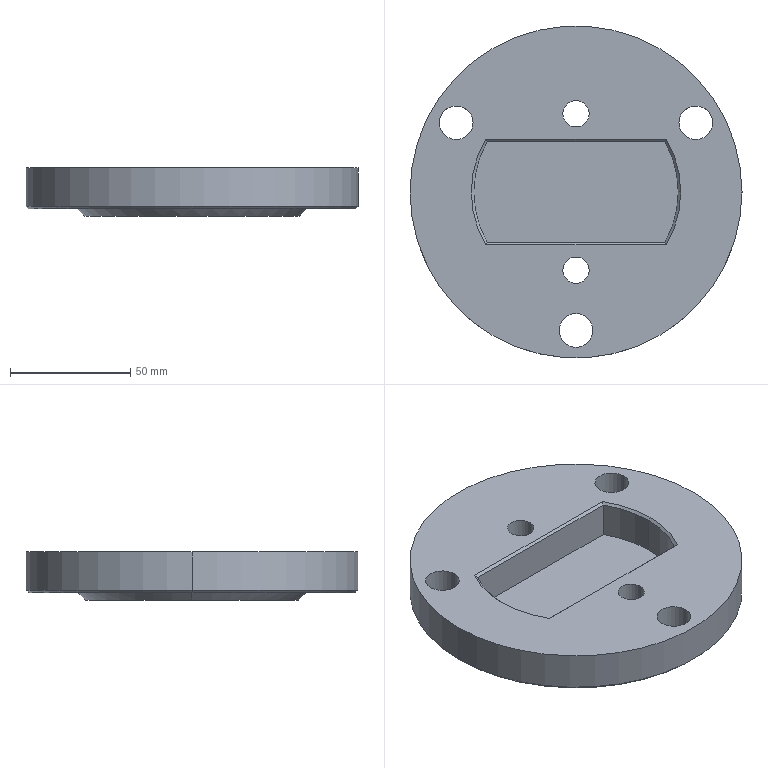Part | SolidWorks | features Chamfer 3, ICE 3, 3DProfileFeature 1, Extrusion 1, HoleWzd 1 | 1 solid | 36 faces | box 138 x 138 x 20 mm | volume 204024 mm3 | cylinder 19 | plane 10 | cone 7 | commonest cylinder face diameters 14 x6 11 x4 18 x4 85 x3 138 x2
STEP:
#1=CARTESIAN_POINT('',(42.5,0.,19.));
#2=VERTEX_POINT('',#1);
#3=CARTESIAN_POINT('',(36.949,21.,19.));
#4=VERTEX_POINT('',#3);
#5=CARTESIAN_POINT('',(0.,0.,19.));
#6=DIRECTION('',(0.,0.,1.));
#7=DIRECTION('',(1.,0.,0.));
#8=AXIS2_PLACEMENT_3D('',#5,#6,#7);
#9=CIRCLE('',#8,42.5);
#10=EDGE_CURVE('',#2,#4,#9,.T.);
#11=ORIENTED_EDGE('',*,*,#10,.F.);
#12=CARTESIAN_POINT('',(43.5,0.,20.));
#13=VERTEX_POINT('',#12);
#14=CARTESIAN_POINT('',(42.5,0.,19.));
#15=DIRECTION('',(0.7071,0.,0.7071));
#16=VECTOR('',#15,1000.);
#17=LINE('',#14,#16);
#18=EDGE_CURVE('',#2,#13,#17,.T.);
#19=ORIENTED_EDGE('',*,*,#18,.T.);
#20=CARTESIAN_POINT('',(37.527,22.,20.));
#21=VERTEX_POINT('',#20);
#22=CARTESIAN_POINT('',(0.,0.,20.));
#23=DIRECTION('',(0.,0.,-1.));
#24=DIRECTION('',(1.,0.,0.));
#25=AXIS2_PLACEMENT_3D('',#22,#23,#24);
#26=CIRCLE('',#25,43.5);
#27=EDGE_CURVE('',#21,#13,#26,.T.);
#28=ORIENTED_EDGE('',*,*,#27,.F.);
#29=CARTESIAN_POINT('',(37.527,22.,20.));
#30=CARTESIAN_POINT('',(37.335,21.666,19.666));
#31=CARTESIAN_POINT('',(37.143,21.333,19.333));
#32=CARTESIAN_POINT('',(36.949,21.,19.));
#33=B_SPLINE_CURVE_WITH_KNOTS('',3,(#29,#30,#31,#32),.UNSPECIFIED.,.F.,.F.,(4,4),(0.,0.001528),.UNSPECIFIED.);
#34=EDGE_CURVE('',#21,#4,#33,.T.);
#35=ORIENTED_EDGE('',*,*,#34,.T.);
#36=EDGE_LOOP('',(#11,#19,#28,#35));
#37=FACE_OUTER_BOUND('',#36,.T.);
#38=CARTESIAN_POINT('',(0.,0.,19.));
#39=DIRECTION('',(0.,0.,1.));
#40=DIRECTION('',(1.,0.,0.));
#41=AXIS2_PLACEMENT_3D('',#38,#39,#40);
#42=CONICAL_SURFACE('',#41,42.5,0.7854);
#43=ADVANCED_FACE('',(#37),#42,.F.);
#44=CARTESIAN_POINT('',(9.,32.5,11.));
#45=VERTEX_POINT('',#44);
#46=CARTESIAN_POINT('',(-9.,32.5,11.));
#47=VERTEX_POINT('',#46);
#48=CARTESIAN_POINT('',(0.,32.5,11.));
#49=DIRECTION('',(0.,0.,-1.));
#50=DIRECTION('',(-1.,0.,0.));
#51=AXIS2_PLACEMENT_3D('',#48,#49,#50);
#52=CIRCLE('',#51,9.);
#53=EDGE_CURVE('',#45,#47,#52,.T.);
#54=ORIENTED_EDGE('',*,*,#53,.F.);
#55=CARTESIAN_POINT('',(9.,32.5,0.));
#56=VERTEX_POINT('',#55);
#57=CARTESIAN_POINT('',(9.,32.5,0.));
#58=DIRECTION('',(0.,0.,-1.));
#59=VECTOR('',#58,1000.);
#60=LINE('',#57,#59);
#61=EDGE_CURVE('',#45,#56,#60,.T.);
#62=ORIENTED_EDGE('',*,*,#61,.T.);
#63=CARTESIAN_POINT('',(-9.,32.5,0.));
#64=VERTEX_POINT('',#63);
#65=CARTESIAN_POINT('',(0.,32.5,0.));
#66=DIRECTION('',(0.,0.,-1.));
#67=DIRECTION('',(-1.,0.,0.));
#68=AXIS2_PLACEMENT_3D('',#65,#66,#67);
#69=CIRCLE('',#68,9.);
#70=EDGE_CURVE('',#56,#64,#69,.T.);
#71=ORIENTED_EDGE('',*,*,#70,.T.);
#72=CARTESIAN_POINT('',(-9.,32.5,0.));
#73=DIRECTION('',(0.,0.,-1.));
#74=VECTOR('',#73,1000.);
#75=LINE('',#72,#74);
#76=EDGE_CURVE('',#47,#64,#75,.T.);
#77=ORIENTED_EDGE('',*,*,#76,.F.);
#78=EDGE_LOOP('',(#54,#62,#71,#77));
#79=FACE_OUTER_BOUND('',#78,.T.);
#80=CARTESIAN_POINT('',(0.,32.5,0.));
#81=DIRECTION('',(0.,0.,-1.));
#82=DIRECTION('',(-1.,0.,0.));
#83=AXIS2_PLACEMENT_3D('',#80,#81,#82);
#84=CYLINDRICAL_SURFACE('',#83,9.);
#85=ADVANCED_FACE('',(#79),#84,.F.);
#86=CARTESIAN_POINT('',(5.5,32.5,20.));
#87=VERTEX_POINT('',#86);
#88=CARTESIAN_POINT('',(-5.5,32.5,20.));
#89=VERTEX_POINT('',#88);
#90=CARTESIAN_POINT('',(0.,32.5,20.));
#91=DIRECTION('',(0.,0.,-1.));
#92=DIRECTION('',(-1.,0.,0.));
#93=AXIS2_PLACEMENT_3D('',#90,#91,#92);
#94=CIRCLE('',#93,5.5);
#95=EDGE_CURVE('',#87,#89,#94,.T.);
#96=ORIENTED_EDGE('',*,*,#95,.F.);
#97=CARTESIAN_POINT('',(5.5,32.5,11.));
#98=VERTEX_POINT('',#97);
#99=CARTESIAN_POINT('',(5.5,32.5,0.));
#100=DIRECTION('',(0.,0.,-1.));
#101=VECTOR('',#100,1000.);
#102=LINE('',#99,#101);
#103=EDGE_CURVE('',#87,#98,#102,.T.);
#104=ORIENTED_EDGE('',*,*,#103,.T.);
#105=CARTESIAN_POINT('',(-5.5,32.5,11.));
#106=VERTEX_POINT('',#105);
#107=CARTESIAN_POINT('',(0.,32.5,11.));
#108=DIRECTION('',(0.,0.,-1.));
#109=DIRECTION('',(-1.,0.,0.));
#110=AXIS2_PLACEMENT_3D('',#107,#108,#109);
#111=CIRCLE('',#110,5.5);
#112=EDGE_CURVE('',#98,#106,#111,.T.);
#113=ORIENTED_EDGE('',*,*,#112,.T.);
#114=CARTESIAN_POINT('',(-5.5,32.5,0.));
#115=DIRECTION('',(0.,0.,-1.));
#116=VECTOR('',#115,1000.);
#117=LINE('',#114,#116);
#118=EDGE_CURVE('',#89,#106,#117,.T.);
#119=ORIENTED_EDGE('',*,*,#118,.F.);
#120=EDGE_LOOP('',(#96,#104,#113,#119));
#121=FACE_OUTER_BOUND('',#120,.T.);
#122=CARTESIAN_POINT('',(0.,32.5,0.));
#123=DIRECTION('',(0.,0.,-1.));
#124=DIRECTION('',(-1.,0.,0.));
#125=AXIS2_PLACEMENT_3D('',#122,#123,#124);
#126=CYLINDRICAL_SURFACE('',#125,5.5);
#127=ADVANCED_FACE('',(#121),#126,.F.);
#128=CARTESIAN_POINT('',(9.,-32.5,11.));
#129=VERTEX_POINT('',#128);
#130=CARTESIAN_POINT('',(-9.,-32.5,11.));
#131=VERTEX_POINT('',#130);
#132=CARTESIAN_POINT('',(0.,-32.5,11.));
#133=DIRECTION('',(0.,0.,-1.));
#134=DIRECTION('',(-1.,0.,0.));
#135=AXIS2_PLACEMENT_3D('',#132,#133,#134);
#136=CIRCLE('',#135,9.);
#137=EDGE_CURVE('',#129,#131,#136,.T.);
#138=ORIENTED_EDGE('',*,*,#137,.F.);
#139=CARTESIAN_POINT('',(9.,-32.5,0.));
#140=VERTEX_POINT('',#139);
#141=CARTESIAN_POINT('',(9.,-32.5,0.));
#142=DIRECTION('',(0.,0.,-1.));
#143=VECTOR('',#142,1000.);
#144=LINE('',#141,#143);
#145=EDGE_CURVE('',#129,#140,#144,.T.);
#146=ORIENTED_EDGE('',*,*,#145,.T.);
#147=CARTESIAN_POINT('',(-9.,-32.5,0.));
#148=VERTEX_POINT('',#147);
#149=CARTESIAN_POINT('',(0.,-32.5,0.));
#150=DIRECTION('',(0.,0.,-1.));
#151=DIRECTION('',(-1.,0.,0.));
#152=AXIS2_PLACEMENT_3D('',#149,#150,#151);
#153=CIRCLE('',#152,9.);
#154=EDGE_CURVE('',#140,#148,#153,.T.);
#155=ORIENTED_EDGE('',*,*,#154,.T.);
#156=CARTESIAN_POINT('',(-9.,-32.5,0.));
#157=DIRECTION('',(0.,0.,-1.));
#158=VECTOR('',#157,1000.);
#159=LINE('',#156,#158);
#160=EDGE_CURVE('',#131,#148,#159,.T.);
#161=ORIENTED_EDGE('',*,*,#160,.F.);
#162=EDGE_LOOP('',(#138,#146,#155,#161));
#163=FACE_OUTER_BOUND('',#162,.T.);
#164=CARTESIAN_POINT('',(0.,-32.5,0.));
#165=DIRECTION('',(0.,0.,-1.));
#166=DIRECTION('',(-1.,0.,0.));
#167=AXIS2_PLACEMENT_3D('',#164,#165,#166);
#168=CYLINDRICAL_SURFACE('',#167,9.);
#169=ADVANCED_FACE('',(#163),#168,.F.);
#170=CARTESIAN_POINT('',(5.5,-32.5,20.));
#171=VERTEX_POINT('',#170);
#172=CARTESIAN_POINT('',(-5.5,-32.5,20.));
#173=VERTEX_POINT('',#172);
#174=CARTESIAN_POINT('',(0.,-32.5,20.));
#175=DIRECTION('',(0.,0.,-1.));
#176=DIRECTION('',(-1.,0.,0.));
#177=AXIS2_PLACEMENT_3D('',#174,#175,#176);
#178=CIRCLE('',#177,5.5);
#179=EDGE_CURVE('',#171,#173,#178,.T.);
#180=ORIENTED_EDGE('',*,*,#179,.F.);
#181=CARTESIAN_POINT('',(5.5,-32.5,11.));
#182=VERTEX_POINT('',#181);
#183=CARTESIAN_POINT('',(5.5,-32.5,0.));
#184=DIRECTION('',(0.,0.,-1.));
#185=VECTOR('',#184,1000.);
#186=LINE('',#183,#185);
#187=EDGE_CURVE('',#171,#182,#186,.T.);
#188=ORIENTED_EDGE('',*,*,#187,.T.);
#189=CARTESIAN_POINT('',(-5.5,-32.5,11.));
#190=VERTEX_POINT('',#189);
#191=CARTESIAN_POINT('',(0.,-32.5,11.));
#192=DIRECTION('',(0.,0.,-1.));
#193=DIRECTION('',(-1.,0.,0.));
#194=AXIS2_PLACEMENT_3D('',#191,#192,#193);
#195=CIRCLE('',#194,5.5);
#196=EDGE_CURVE('',#182,#190,#195,.T.);
#197=ORIENTED_EDGE('',*,*,#196,.T.);
#198=CARTESIAN_POINT('',(-5.5,-32.5,0.));
#199=DIRECTION('',(0.,0.,-1.));
#200=VECTOR('',#199,1000.);
#201=LINE('',#198,#200);
#202=EDGE_CURVE('',#173,#190,#201,.T.);
#203=ORIENTED_EDGE('',*,*,#202,.F.);
#204=EDGE_LOOP('',(#180,#188,#197,#203));
#205=FACE_OUTER_BOUND('',#204,.T.);
#206=CARTESIAN_POINT('',(0.,-32.5,0.));
#207=DIRECTION('',(0.,0.,-1.));
#208=DIRECTION('',(-1.,0.,0.));
#209=AXIS2_PLACEMENT_3D('',#206,#207,#208);
#210=CYLINDRICAL_SURFACE('',#209,5.5);
#211=ADVANCED_FACE('',(#205),#210,.F.);
#212=CARTESIAN_POINT('',(-44.5,0.,0.));
#213=VERTEX_POINT('',#212);
#214=CARTESIAN_POINT('',(44.5,0.,0.));
#215=VERTEX_POINT('',#214);
#216=CARTESIAN_POINT('',(0.,0.,0.));
#217=DIRECTION('',(0.,0.,-1.));
#218=DIRECTION('',(1.,0.,0.));
#219=AXIS2_PLACEMENT_3D('',#216,#217,#218);
#220=CIRCLE('',#219,44.5);
#221=EDGE_CURVE('',#213,#215,#220,.T.);
#222=ORIENTED_EDGE('',*,*,#221,.F.);
#223=CARTESIAN_POINT('',(-47.5,0.,3.));
#224=VERTEX_POINT('',#223);
#225=CARTESIAN_POINT('',(-44.5,0.,0.));
#226=DIRECTION('',(-0.7071,0.,0.7071));
#227=VECTOR('',#226,1000.);
#228=LINE('',#225,#227);
#229=EDGE_CURVE('',#213,#224,#228,.T.);
#230=ORIENTED_EDGE('',*,*,#229,.T.);
#231=CARTESIAN_POINT('',(47.5,0.,3.));
#232=VERTEX_POINT('',#231);
#233=CARTESIAN_POINT('',(0.,0.,3.));
#234=DIRECTION('',(0.,0.,-1.));
#235=DIRECTION('',(-1.,0.,0.));
#236=AXIS2_PLACEMENT_3D('',#233,#234,#235);
#237=CIRCLE('',#236,47.5);
#238=EDGE_CURVE('',#224,#232,#237,.T.);
#239=ORIENTED_EDGE('',*,*,#238,.T.);
#240=CARTESIAN_POINT('',(44.5,0.,0.));
#241=DIRECTION('',(0.7071,0.,0.7071));
#242=VECTOR('',#241,1000.);
#243=LINE('',#240,#242);
#244=EDGE_CURVE('',#215,#232,#243,.T.);
#245=ORIENTED_EDGE('',*,*,#244,.F.);
#246=EDGE_LOOP('',(#222,#230,#239,#245));
#247=FACE_OUTER_BOUND('',#246,.T.);
#248=CARTESIAN_POINT('',(0.,0.,0.));
#249=DIRECTION('',(0.,0.,1.));
#250=DIRECTION('',(1.,0.,0.));
#251=AXIS2_PLACEMENT_3D('',#248,#249,#250);
#252=CONICAL_SURFACE('',#251,44.5,0.7854);
#253=ADVANCED_FACE('',(#247),#252,.T.);
#254=CARTESIAN_POINT('',(-68.,0.,3.));
#255=VERTEX_POINT('',#254);
#256=CARTESIAN_POINT('',(68.,0.,3.));
#257=VERTEX_POINT('',#256);
#258=CARTESIAN_POINT('',(0.,0.,3.));
#259=DIRECTION('',(0.,0.,-1.));
#260=DIRECTION('',(-1.,0.,0.));
#261=AXIS2_PLACEMENT_3D('',#258,#259,#260);
#262=CIRCLE('',#261,68.);
#263=EDGE_CURVE('',#255,#257,#262,.T.);
#264=ORIENTED_EDGE('',*,*,#263,.F.);
#265=CARTESIAN_POINT('',(-69.,0.,4.));
#266=VERTEX_POINT('',#265);
#267=CARTESIAN_POINT('',(-68.,0.,3.));
#268=DIRECTION('',(-0.7071,0.,0.7071));
#269=VECTOR('',#268,1000.);
#270=LINE('',#267,#269);
#271=EDGE_CURVE('',#255,#266,#270,.T.);
#272=ORIENTED_EDGE('',*,*,#271,.T.);
#273=CARTESIAN_POINT('',(69.,0.,4.));
#274=VERTEX_POINT('',#273);
#275=CARTESIAN_POINT('',(0.,0.,4.));
#276=DIRECTION('',(0.,0.,1.));
#277=DIRECTION('',(-1.,0.,0.));
#278=AXIS2_PLACEMENT_3D('',#275,#276,#277);
#279=CIRCLE('',#278,69.);
#280=EDGE_CURVE('',#274,#266,#279,.T.);
#281=ORIENTED_EDGE('',*,*,#280,.F.);
#282=CARTESIAN_POINT('',(68.,0.,3.));
#283=DIRECTION('',(0.7071,0.,0.7071));
#284=VECTOR('',#283,1000.);
#285=LINE('',#282,#284);
#286=EDGE_CURVE('',#257,#274,#285,.T.);
#287=ORIENTED_EDGE('',*,*,#286,.F.);
#288=EDGE_LOOP('',(#264,#272,#281,#287));
#289=FACE_OUTER_BOUND('',#288,.T.);
#290=CARTESIAN_POINT('',(0.,0.,3.));
#291=DIRECTION('',(0.,0.,1.));
#292=DIRECTION('',(1.,0.,0.));
#293=AXIS2_PLACEMENT_3D('',#290,#291,#292);
#294=CONICAL_SURFACE('',#293,68.,0.7854);
#295=ADVANCED_FACE('',(#289),#294,.T.);
#296=CARTESIAN_POINT('',(56.796,28.75,20.));
#297=VERTEX_POINT('',#296);
#298=CARTESIAN_POINT('',(42.796,28.75,20.));
#299=VERTEX_POINT('',#298);
#300=CARTESIAN_POINT('',(49.796,28.75,20.));
#301=DIRECTION('',(0.,0.,-1.));
#302=DIRECTION('',(-1.,0.,0.));
#303=AXIS2_PLACEMENT_3D('',#300,#301,#302);
#304=CIRCLE('',#303,7.);
#305=EDGE_CURVE('',#297,#299,#304,.T.);
#306=ORIENTED_EDGE('',*,*,#305,.F.);
#307=CARTESIAN_POINT('',(56.796,28.75,3.));
#308=VERTEX_POINT('',#307);
#309=CARTESIAN_POINT('',(56.796,28.75,20.));
#310=DIRECTION('',(0.,0.,-1.));
#311=VECTOR('',#310,1000.);
#312=LINE('',#309,#311);
#313=EDGE_CURVE('',#297,#308,#312,.T.);
#314=ORIENTED_EDGE('',*,*,#313,.T.);
#315=CARTESIAN_POINT('',(42.796,28.75,3.));
#316=VERTEX_POINT('',#315);
#317=CARTESIAN_POINT('',(49.796,28.75,3.));
#318=DIRECTION('',(0.,0.,-1.));
#319=DIRECTION('',(-1.,0.,0.));
#320=AXIS2_PLACEMENT_3D('',#317,#318,#319);
#321=CIRCLE('',#320,7.);
#322=EDGE_CURVE('',#308,#316,#321,.T.);
#323=ORIENTED_EDGE('',*,*,#322,.T.);
#324=CARTESIAN_POINT('',(42.796,28.75,20.));
#325=DIRECTION('',(0.,0.,-1.));
#326=VECTOR('',#325,1000.);
#327=LINE('',#324,#326);
#328=EDGE_CURVE('',#299,#316,#327,.T.);
#329=ORIENTED_EDGE('',*,*,#328,.F.);
#330=EDGE_LOOP('',(#306,#314,#323,#329));
#331=FACE_OUTER_BOUND('',#330,.T.);
#332=CARTESIAN_POINT('',(49.796,28.75,20.));
#333=DIRECTION('',(0.,0.,-1.));
#334=DIRECTION('',(-1.,0.,0.));
#335=AXIS2_PLACEMENT_3D('',#332,#333,#334);
#336=CYLINDRICAL_SURFACE('',#335,7.);
#337=ADVANCED_FACE('',(#331),#336,.F.);
#338=CARTESIAN_POINT('',(-42.796,28.75,20.));
#339=VERTEX_POINT('',#338);
#340=CARTESIAN_POINT('',(-56.796,28.75,20.));
#341=VERTEX_POINT('',#340);
#342=CARTESIAN_POINT('',(-49.796,28.75,20.));
#343=DIRECTION('',(0.,0.,-1.));
#344=DIRECTION('',(-1.,0.,0.));
#345=AXIS2_PLACEMENT_3D('',#342,#343,#344);
#346=CIRCLE('',#345,7.);
#347=EDGE_CURVE('',#339,#341,#346,.T.);
#348=ORIENTED_EDGE('',*,*,#347,.F.);
#349=CARTESIAN_POINT('',(-42.796,28.75,3.));
#350=VERTEX_POINT('',#349);
#351=CARTESIAN_POINT('',(-42.796,28.75,20.));
#352=DIRECTION('',(0.,0.,-1.));
#353=VECTOR('',#352,1000.);
#354=LINE('',#351,#353);
#355=EDGE_CURVE('',#339,#350,#354,.T.);
#356=ORIENTED_EDGE('',*,*,#355,.T.);
#357=CARTESIAN_POINT('',(-56.796,28.75,3.));
#358=VERTEX_POINT('',#357);
#359=CARTESIAN_POINT('',(-49.796,28.75,3.));
#360=DIRECTION('',(0.,0.,-1.));
#361=DIRECTION('',(-1.,0.,0.));
#362=AXIS2_PLACEMENT_3D('',#359,#360,#361);
#363=CIRCLE('',#362,7.);
#364=EDGE_CURVE('',#350,#358,#363,.T.);
#365=ORIENTED_EDGE('',*,*,#364,.T.);
#366=CARTESIAN_POINT('',(-56.796,28.75,20.));
#367=DIRECTION('',(0.,0.,-1.));
#368=VECTOR('',#367,1000.);
#369=LINE('',#366,#368);
#370=EDGE_CURVE('',#341,#358,#369,.T.);
#371=ORIENTED_EDGE('',*,*,#370,.F.);
#372=EDGE_LOOP('',(#348,#356,#365,#371));
#373=FACE_OUTER_BOUND('',#372,.T.);
#374=CARTESIAN_POINT('',(-49.796,28.75,20.));
#375=DIRECTION('',(0.,0.,-1.));
#376=DIRECTION('',(-1.,0.,0.));
#377=AXIS2_PLACEMENT_3D('',#374,#375,#376);
#378=CYLINDRICAL_SURFACE('',#377,7.);
#379=ADVANCED_FACE('',(#373),#378,.F.);
#380=CARTESIAN_POINT('',(7.,-57.5,20.));
#381=VERTEX_POINT('',#380);
#382=CARTESIAN_POINT('',(-7.,-57.5,20.));
#383=VERTEX_POINT('',#382);
#384=CARTESIAN_POINT('',(0.,-57.5,20.));
#385=DIRECTION('',(0.,0.,-1.));
#386=DIRECTION('',(-1.,0.,0.));
#387=AXIS2_PLACEMENT_3D('',#384,#385,#386);
#388=CIRCLE('',#387,7.);
#389=EDGE_CURVE('',#381,#383,#388,.T.);
#390=ORIENTED_EDGE('',*,*,#389,.F.);
#391=CARTESIAN_POINT('',(7.,-57.5,3.));
#392=VERTEX_POINT('',#391);
#393=CARTESIAN_POINT('',(7.,-57.5,20.));
#394=DIRECTION('',(0.,0.,-1.));
#395=VECTOR('',#394,1000.);
#396=LINE('',#393,#395);
#397=EDGE_CURVE('',#381,#392,#396,.T.);
#398=ORIENTED_EDGE('',*,*,#397,.T.);
#399=CARTESIAN_POINT('',(-7.,-57.5,3.));
#400=VERTEX_POINT('',#399);
#401=CARTESIAN_POINT('',(0.,-57.5,3.));
#402=DIRECTION('',(0.,0.,-1.));
#403=DIRECTION('',(-1.,0.,0.));
#404=AXIS2_PLACEMENT_3D('',#401,#402,#403);
#405=CIRCLE('',#404,7.);
#406=EDGE_CURVE('',#392,#400,#405,.T.);
#407=ORIENTED_EDGE('',*,*,#406,.T.);
#408=CARTESIAN_POINT('',(-7.,-57.5,20.));
#409=DIRECTION('',(0.,0.,-1.));
#410=VECTOR('',#409,1000.);
#411=LINE('',#408,#410);
#412=EDGE_CURVE('',#383,#400,#411,.T.);
#413=ORIENTED_EDGE('',*,*,#412,.F.);
#414=EDGE_LOOP('',(#390,#398,#407,#413));
#415=FACE_OUTER_BOUND('',#414,.T.);
#416=CARTESIAN_POINT('',(0.,-57.5,20.));
#417=DIRECTION('',(0.,0.,-1.));
#418=DIRECTION('',(-1.,0.,0.));
#419=AXIS2_PLACEMENT_3D('',#416,#417,#418);
#420=CYLINDRICAL_SURFACE('',#419,7.);
#421=ADVANCED_FACE('',(#415),#420,.F.);
#422=CARTESIAN_POINT('',(42.5,0.,4.));
#423=VERTEX_POINT('',#422);
#424=CARTESIAN_POINT('',(36.949,21.,4.));
#425=VERTEX_POINT('',#424);
#426=CARTESIAN_POINT('',(0.,0.,4.));
#427=DIRECTION('',(0.,0.,1.));
#428=DIRECTION('',(1.,0.,0.));
#429=AXIS2_PLACEMENT_3D('',#426,#427,#428);
#430=CIRCLE('',#429,42.5);
#431=EDGE_CURVE('',#423,#425,#430,.T.);
#432=ORIENTED_EDGE('',*,*,#431,.F.);
#433=CARTESIAN_POINT('',(42.5,0.,4.));
#434=DIRECTION('',(0.,0.,1.));
#435=VECTOR('',#434,1000.);
#436=LINE('',#433,#435);
#437=EDGE_CURVE('',#423,#2,#436,.T.);
#438=ORIENTED_EDGE('',*,*,#437,.T.);
#439=ORIENTED_EDGE('',*,*,#10,.T.);
#440=CARTESIAN_POINT('',(36.949,21.,4.));
#441=DIRECTION('',(0.,0.,1.));
#442=VECTOR('',#441,1000.);
#443=LINE('',#440,#442);
#444=EDGE_CURVE('',#425,#4,#443,.T.);
#445=ORIENTED_EDGE('',*,*,#444,.F.);
#446=EDGE_LOOP('',(#432,#438,#439,#445));
#447=FACE_OUTER_BOUND('',#446,.T.);
#448=CARTESIAN_POINT('',(0.,0.,4.));
#449=DIRECTION('',(0.,0.,1.));
#450=DIRECTION('',(1.,0.,0.));
#451=AXIS2_PLACEMENT_3D('',#448,#449,#450);
#452=CYLINDRICAL_SURFACE('',#451,42.5);
#453=ADVANCED_FACE('',(#447),#452,.F.);
#454=CARTESIAN_POINT('',(69.,0.,20.));
#455=VERTEX_POINT('',#454);
#456=CARTESIAN_POINT('',(-69.,0.,20.));
#457=VERTEX_POINT('',#456);
#458=CARTESIAN_POINT('',(0.,0.,20.));
#459=DIRECTION('',(0.,0.,1.));
#460=DIRECTION('',(1.,0.,0.));
#461=AXIS2_PLACEMENT_3D('',#458,#459,#460);
#462=CIRCLE('',#461,69.);
#463=EDGE_CURVE('',#455,#457,#462,.T.);
#464=ORIENTED_EDGE('',*,*,#463,.F.);
#465=CARTESIAN_POINT('',(69.,0.,20.));
#466=DIRECTION('',(0.,0.,-1.));
#467=VECTOR('',#466,1000.);
#468=LINE('',#465,#467);
#469=EDGE_CURVE('',#455,#274,#468,.T.);
#470=ORIENTED_EDGE('',*,*,#469,.T.);
#471=ORIENTED_EDGE('',*,*,#280,.T.);
#472=CARTESIAN_POINT('',(-69.,0.,20.));
#473=DIRECTION('',(0.,0.,-1.));
#474=VECTOR('',#473,1000.);
#475=LINE('',#472,#474);
#476=EDGE_CURVE('',#457,#266,#475,.T.);
#477=ORIENTED_EDGE('',*,*,#476,.F.);
#478=EDGE_LOOP('',(#464,#470,#471,#477));
#479=FACE_OUTER_BOUND('',#478,.T.);
#480=CARTESIAN_POINT('',(0.,0.,20.));
#481=DIRECTION('',(0.,0.,-1.));
#482=DIRECTION('',(-1.,0.,0.));
#483=AXIS2_PLACEMENT_3D('',#480,#481,#482);
#484=CYLINDRICAL_SURFACE('',#483,69.);
#485=ADVANCED_FACE('',(#479),#484,.T.);
#486=ORIENTED_EDGE('',*,*,#469,.F.);
#487=CARTESIAN_POINT('',(0.,0.,20.));
#488=DIRECTION('',(0.,0.,1.));
#489=DIRECTION('',(1.,0.,0.));
#490=AXIS2_PLACEMENT_3D('',#487,#488,#489);
#491=CIRCLE('',#490,69.);
#492=EDGE_CURVE('',#457,#455,#491,.T.);
#493=ORIENTED_EDGE('',*,*,#492,.F.);
#494=ORIENTED_EDGE('',*,*,#476,.T.);
#495=CARTESIAN_POINT('',(0.,0.,4.));
#496=DIRECTION('',(0.,0.,1.));
#497=DIRECTION('',(-1.,0.,0.));
#498=AXIS2_PLACEMENT_3D('',#495,#496,#497);
#499=CIRCLE('',#498,69.);
#500=EDGE_CURVE('',#266,#274,#499,.T.);
#501=ORIENTED_EDGE('',*,*,#500,.T.);
#502=EDGE_LOOP('',(#486,#493,#494,#501));
#503=FACE_OUTER_BOUND('',#502,.T.);
#504=CARTESIAN_POINT('',(0.,0.,20.));
#505=DIRECTION('',(0.,0.,-1.));
#506=DIRECTION('',(-1.,0.,0.));
#507=AXIS2_PLACEMENT_3D('',#504,#505,#506);
#508=CYLINDRICAL_SURFACE('',#507,69.);
#509=ADVANCED_FACE('',(#503),#508,.T.);
#510=CARTESIAN_POINT('',(-37.527,22.,20.));
#511=VERTEX_POINT('',#510);
#512=CARTESIAN_POINT('',(36.949,22.,20.));
#513=DIRECTION('',(1.,0.,0.));
#514=VECTOR('',#513,1000.);
#515=LINE('',#512,#514);
#516=EDGE_CURVE('',#511,#21,#515,.T.);
#517=ORIENTED_EDGE('',*,*,#516,.T.);
#518=ORIENTED_EDGE('',*,*,#27,.T.);
#519=CARTESIAN_POINT('',(37.527,-22.,20.));
#520=VERTEX_POINT('',#519);
#521=CARTESIAN_POINT('',(0.,0.,20.));
#522=DIRECTION('',(0.,0.,-1.));
#523=DIRECTION('',(1.,0.,0.));
#524=AXIS2_PLACEMENT_3D('',#521,#522,#523);
#525=CIRCLE('',#524,43.5);
#526=EDGE_CURVE('',#13,#520,#525,.T.);
#527=ORIENTED_EDGE('',*,*,#526,.T.);
#528=CARTESIAN_POINT('',(-37.527,-22.,20.));
#529=VERTEX_POINT('',#528);
#530=CARTESIAN_POINT('',(-36.949,-22.,20.));
#531=DIRECTION('',(-1.,0.,0.));
#532=VECTOR('',#531,1000.);
#533=LINE('',#530,#532);
#534=EDGE_CURVE('',#520,#529,#533,.T.);
#535=ORIENTED_EDGE('',*,*,#534,.T.);
#536=CARTESIAN_POINT('',(0.,0.,20.));
#537=DIRECTION('',(0.,0.,-1.));
#538=DIRECTION('',(1.,0.,0.));
#539=AXIS2_PLACEMENT_3D('',#536,#537,#538);
#540=CIRCLE('',#539,43.5);
#541=EDGE_CURVE('',#529,#511,#540,.T.);
#542=ORIENTED_EDGE('',*,*,#541,.T.);
#543=EDGE_LOOP('',(#517,#518,#527,#535,#542));
#544=FACE_BOUND('',#543,.T.);
#545=CARTESIAN_POINT('',(0.,32.5,20.));
#546=DIRECTION('',(0.,0.,-1.));
#547=DIRECTION('',(-1.,0.,0.));
#548=AXIS2_PLACEMENT_3D('',#545,#546,#547);
#549=CIRCLE('',#548,5.5);
#550=EDGE_CURVE('',#89,#87,#549,.T.);
#551=ORIENTED_EDGE('',*,*,#550,.T.);
#552=ORIENTED_EDGE('',*,*,#95,.T.);
#553=EDGE_LOOP('',(#551,#552));
#554=FACE_BOUND('',#553,.T.);
#555=CARTESIAN_POINT('',(0.,-32.5,20.));
#556=DIRECTION('',(0.,0.,-1.));
#557=DIRECTION('',(-1.,0.,0.));
#558=AXIS2_PLACEMENT_3D('',#555,#556,#557);
#559=CIRCLE('',#558,5.5);
#560=EDGE_CURVE('',#173,#171,#559,.T.);
#561=ORIENTED_EDGE('',*,*,#560,.T.);
#562=ORIENTED_EDGE('',*,*,#179,.T.);
#563=EDGE_LOOP('',(#561,#562));
#564=FACE_BOUND('',#563,.T.);
#565=CARTESIAN_POINT('',(49.796,28.75,20.));
#566=DIRECTION('',(0.,0.,-1.));
#567=DIRECTION('',(-1.,0.,0.));
#568=AXIS2_PLACEMENT_3D('',#565,#566,#567);
#569=CIRCLE('',#568,7.);
#570=EDGE_CURVE('',#299,#297,#569,.T.);
#571=ORIENTED_EDGE('',*,*,#570,.T.);
#572=ORIENTED_EDGE('',*,*,#305,.T.);
#573=EDGE_LOOP('',(#571,#572));
#574=FACE_BOUND('',#573,.T.);
#575=CARTESIAN_POINT('',(-49.796,28.75,20.));
#576=DIRECTION('',(0.,0.,-1.));
#577=DIRECTION('',(-1.,0.,0.));
#578=AXIS2_PLACEMENT_3D('',#575,#576,#577);
#579=CIRCLE('',#578,7.);
#580=EDGE_CURVE('',#341,#339,#579,.T.);
#581=ORIENTED_EDGE('',*,*,#580,.T.);
#582=ORIENTED_EDGE('',*,*,#347,.T.);
#583=EDGE_LOOP('',(#581,#582));
#584=FACE_BOUND('',#583,.T.);
#585=CARTESIAN_POINT('',(0.,-57.5,20.));
#586=DIRECTION('',(0.,0.,-1.));
#587=DIRECTION('',(-1.,0.,0.));
#588=AXIS2_PLACEMENT_3D('',#585,#586,#587);
#589=CIRCLE('',#588,7.);
#590=EDGE_CURVE('',#383,#381,#589,.T.);
#591=ORIENTED_EDGE('',*,*,#590,.T.);
#592=ORIENTED_EDGE('',*,*,#389,.T.);
#593=EDGE_LOOP('',(#591,#592));
#594=FACE_BOUND('',#593,.T.);
#595=ORIENTED_EDGE('',*,*,#492,.T.);
#596=ORIENTED_EDGE('',*,*,#463,.T.);
#597=EDGE_LOOP('',(#595,#596));
#598=FACE_OUTER_BOUND('',#597,.T.);
#599=CARTESIAN_POINT('',(0.,0.,20.));
#600=DIRECTION('',(0.,0.,1.));
#601=DIRECTION('',(1.,0.,0.));
#602=AXIS2_PLACEMENT_3D('',#599,#600,#601);
#603=PLANE('',#602);
#604=ADVANCED_FACE('',(#544,#554,#564,#574,#584,#594,#598),#603,.T.);
#605=CARTESIAN_POINT('',(-36.949,21.,4.));
#606=VERTEX_POINT('',#605);
#607=CARTESIAN_POINT('',(-36.949,21.,19.));
#608=VERTEX_POINT('',#607);
#609=CARTESIAN_POINT('',(-36.949,21.,4.));
#610=DIRECTION('',(0.,0.,1.));
#611=VECTOR('',#610,1000.);
#612=LINE('',#609,#611);
#613=EDGE_CURVE('',#606,#608,#612,.T.);
#614=ORIENTED_EDGE('',*,*,#613,.T.);
#615=CARTESIAN_POINT('',(-36.949,-21.,19.));
#616=VERTEX_POINT('',#615);
#617=CARTESIAN_POINT('',(0.,0.,19.));
#618=DIRECTION('',(0.,0.,1.));
#619=DIRECTION('',(1.,0.,0.));
#620=AXIS2_PLACEMENT_3D('',#617,#618,#619);
#621=CIRCLE('',#620,42.5);
#622=EDGE_CURVE('',#608,#616,#621,.T.);
#623=ORIENTED_EDGE('',*,*,#622,.T.);
#624=CARTESIAN_POINT('',(-36.949,-21.,4.));
#625=VERTEX_POINT('',#624);
#626=CARTESIAN_POINT('',(-36.949,-21.,4.));
#627=DIRECTION('',(0.,0.,1.));
#628=VECTOR('',#627,1000.);
#629=LINE('',#626,#628);
#630=EDGE_CURVE('',#625,#616,#629,.T.);
#631=ORIENTED_EDGE('',*,*,#630,.F.);
#632=CARTESIAN_POINT('',(0.,0.,4.));
#633=DIRECTION('',(0.,0.,1.));
#634=DIRECTION('',(1.,0.,0.));
#635=AXIS2_PLACEMENT_3D('',#632,#633,#634);
#636=CIRCLE('',#635,42.5);
#637=EDGE_CURVE('',#606,#625,#636,.T.);
#638=ORIENTED_EDGE('',*,*,#637,.F.);
#639=EDGE_LOOP('',(#614,#623,#631,#638));
#640=FACE_OUTER_BOUND('',#639,.T.);
#641=CARTESIAN_POINT('',(0.,0.,4.));
#642=DIRECTION('',(0.,0.,1.));
#643=DIRECTION('',(1.,0.,0.));
#644=AXIS2_PLACEMENT_3D('',#641,#642,#643);
#645=CYLINDRICAL_SURFACE('',#644,42.5);
#646=ADVANCED_FACE('',(#640),#645,.F.);
#647=ORIENTED_EDGE('',*,*,#444,.T.);
#648=CARTESIAN_POINT('',(-36.949,21.,19.));
#649=DIRECTION('',(-1.,0.,0.));
#650=VECTOR('',#649,1000.);
#651=LINE('',#648,#650);
#652=EDGE_CURVE('',#4,#608,#651,.T.);
#653=ORIENTED_EDGE('',*,*,#652,.T.);
#654=ORIENTED_EDGE('',*,*,#613,.F.);
#655=CARTESIAN_POINT('',(-36.949,21.,4.));
#656=DIRECTION('',(-1.,0.,0.));
#657=VECTOR('',#656,1000.);
#658=LINE('',#655,#657);
#659=EDGE_CURVE('',#425,#606,#658,.T.);
#660=ORIENTED_EDGE('',*,*,#659,.F.);
#661=EDGE_LOOP('',(#647,#653,#654,#660));
#662=FACE_OUTER_BOUND('',#661,.T.);
#663=CARTESIAN_POINT('',(-36.949,21.,4.));
#664=DIRECTION('',(0.,1.,0.));
#665=DIRECTION('',(0.,0.,1.));
#666=AXIS2_PLACEMENT_3D('',#663,#664,#665);
#667=PLANE('',#666);
#668=ADVANCED_FACE('',(#662),#667,.F.);
#669=ORIENTED_EDGE('',*,*,#437,.F.);
#670=CARTESIAN_POINT('',(36.949,-21.,4.));
#671=VERTEX_POINT('',#670);
#672=CARTESIAN_POINT('',(0.,0.,4.));
#673=DIRECTION('',(0.,0.,1.));
#674=DIRECTION('',(1.,0.,0.));
#675=AXIS2_PLACEMENT_3D('',#672,#673,#674);
#676=CIRCLE('',#675,42.5);
#677=EDGE_CURVE('',#671,#423,#676,.T.);
#678=ORIENTED_EDGE('',*,*,#677,.F.);
#679=CARTESIAN_POINT('',(36.949,-21.,19.));
#680=VERTEX_POINT('',#679);
#681=CARTESIAN_POINT('',(36.949,-21.,4.));
#682=DIRECTION('',(0.,0.,1.));
#683=VECTOR('',#682,1000.);
#684=LINE('',#681,#683);
#685=EDGE_CURVE('',#671,#680,#684,.T.);
#686=ORIENTED_EDGE('',*,*,#685,.T.);
#687=CARTESIAN_POINT('',(0.,0.,19.));
#688=DIRECTION('',(0.,0.,1.));
#689=DIRECTION('',(1.,0.,0.));
#690=AXIS2_PLACEMENT_3D('',#687,#688,#689);
#691=CIRCLE('',#690,42.5);
#692=EDGE_CURVE('',#680,#2,#691,.T.);
#693=ORIENTED_EDGE('',*,*,#692,.T.);
#694=EDGE_LOOP('',(#669,#678,#686,#693));
#695=FACE_OUTER_BOUND('',#694,.T.);
#696=CARTESIAN_POINT('',(0.,0.,4.));
#697=DIRECTION('',(0.,0.,1.));
#698=DIRECTION('',(1.,0.,0.));
#699=AXIS2_PLACEMENT_3D('',#696,#697,#698);
#700=CYLINDRICAL_SURFACE('',#699,42.5);
#701=ADVANCED_FACE('',(#695),#700,.F.);
#702=ORIENTED_EDGE('',*,*,#630,.T.);
#703=CARTESIAN_POINT('',(36.949,-21.,19.));
#704=DIRECTION('',(1.,0.,0.));
#705=VECTOR('',#704,1000.);
#706=LINE('',#703,#705);
#707=EDGE_CURVE('',#616,#680,#706,.T.);
#708=ORIENTED_EDGE('',*,*,#707,.T.);
#709=ORIENTED_EDGE('',*,*,#685,.F.);
#710=CARTESIAN_POINT('',(-36.949,-21.,4.));
#711=DIRECTION('',(1.,0.,0.));
#712=VECTOR('',#711,1000.);
#713=LINE('',#710,#712);
#714=EDGE_CURVE('',#625,#671,#713,.T.);
#715=ORIENTED_EDGE('',*,*,#714,.F.);
#716=EDGE_LOOP('',(#702,#708,#709,#715));
#717=FACE_OUTER_BOUND('',#716,.T.);
#718=CARTESIAN_POINT('',(-36.949,-21.,4.));
#719=DIRECTION('',(0.,-1.,0.));
#720=DIRECTION('',(0.,0.,-1.));
#721=AXIS2_PLACEMENT_3D('',#718,#719,#720);
#722=PLANE('',#721);
#723=ADVANCED_FACE('',(#717),#722,.F.);
#724=ORIENTED_EDGE('',*,*,#637,.T.);
#725=ORIENTED_EDGE('',*,*,#714,.T.);
#726=ORIENTED_EDGE('',*,*,#677,.T.);
#727=ORIENTED_EDGE('',*,*,#431,.T.);
#728=ORIENTED_EDGE('',*,*,#659,.T.);
#729=EDGE_LOOP('',(#724,#725,#726,#727,#728));
#730=FACE_OUTER_BOUND('',#729,.T.);
#731=CARTESIAN_POINT('',(0.,0.,4.));
#732=DIRECTION('',(0.,0.,1.));
#733=DIRECTION('',(1.,0.,0.));
#734=AXIS2_PLACEMENT_3D('',#731,#732,#733);
#735=PLANE('',#734);
#736=ADVANCED_FACE('',(#730),#735,.T.);
#737=CARTESIAN_POINT('',(0.,0.,3.));
#738=DIRECTION('',(0.,0.,-1.));
#739=DIRECTION('',(-1.,0.,0.));
#740=AXIS2_PLACEMENT_3D('',#737,#738,#739);
#741=CIRCLE('',#740,68.);
#742=EDGE_CURVE('',#257,#255,#741,.T.);
#743=ORIENTED_EDGE('',*,*,#742,.T.);
#744=ORIENTED_EDGE('',*,*,#263,.T.);
#745=EDGE_LOOP('',(#743,#744));
#746=FACE_OUTER_BOUND('',#745,.T.);
#747=CARTESIAN_POINT('',(49.796,28.75,3.));
#748=DIRECTION('',(0.,0.,-1.));
#749=DIRECTION('',(-1.,0.,0.));
#750=AXIS2_PLACEMENT_3D('',#747,#748,#749);
#751=CIRCLE('',#750,7.);
#752=EDGE_CURVE('',#316,#308,#751,.T.);
#753=ORIENTED_EDGE('',*,*,#752,.F.);
#754=ORIENTED_EDGE('',*,*,#322,.F.);
#755=EDGE_LOOP('',(#753,#754));
#756=FACE_BOUND('',#755,.T.);
#757=CARTESIAN_POINT('',(-49.796,28.75,3.));
#758=DIRECTION('',(0.,0.,-1.));
#759=DIRECTION('',(-1.,0.,0.));
#760=AXIS2_PLACEMENT_3D('',#757,#758,#759);
#761=CIRCLE('',#760,7.);
#762=EDGE_CURVE('',#358,#350,#761,.T.);
#763=ORIENTED_EDGE('',*,*,#762,.F.);
#764=ORIENTED_EDGE('',*,*,#364,.F.);
#765=EDGE_LOOP('',(#763,#764));
#766=FACE_BOUND('',#765,.T.);
#767=CARTESIAN_POINT('',(0.,-57.5,3.));
#768=DIRECTION('',(0.,0.,-1.));
#769=DIRECTION('',(-1.,0.,0.));
#770=AXIS2_PLACEMENT_3D('',#767,#768,#769);
#771=CIRCLE('',#770,7.);
#772=EDGE_CURVE('',#400,#392,#771,.T.);
#773=ORIENTED_EDGE('',*,*,#772,.F.);
#774=ORIENTED_EDGE('',*,*,#406,.F.);
#775=EDGE_LOOP('',(#773,#774));
#776=FACE_BOUND('',#775,.T.);
#777=CARTESIAN_POINT('',(0.,0.,3.));
#778=DIRECTION('',(0.,0.,-1.));
#779=DIRECTION('',(-1.,0.,0.));
#780=AXIS2_PLACEMENT_3D('',#777,#778,#779);
#781=CIRCLE('',#780,47.5);
#782=EDGE_CURVE('',#232,#224,#781,.T.);
#783=ORIENTED_EDGE('',*,*,#782,.F.);
#784=ORIENTED_EDGE('',*,*,#238,.F.);
#785=EDGE_LOOP('',(#783,#784));
#786=FACE_BOUND('',#785,.T.);
#787=CARTESIAN_POINT('',(0.,0.,3.));
#788=DIRECTION('',(0.,0.,-1.));
#789=DIRECTION('',(-1.,0.,0.));
#790=AXIS2_PLACEMENT_3D('',#787,#788,#789);
#791=PLANE('',#790);
#792=ADVANCED_FACE('',(#746,#756,#766,#776,#786),#791,.T.);
#793=CARTESIAN_POINT('',(0.,32.5,0.));
#794=DIRECTION('',(0.,0.,-1.));
#795=DIRECTION('',(-1.,0.,0.));
#796=AXIS2_PLACEMENT_3D('',#793,#794,#795);
#797=CIRCLE('',#796,9.);
#798=EDGE_CURVE('',#64,#56,#797,.T.);
#799=ORIENTED_EDGE('',*,*,#798,.F.);
#800=ORIENTED_EDGE('',*,*,#70,.F.);
#801=EDGE_LOOP('',(#799,#800));
#802=FACE_BOUND('',#801,.T.);
#803=CARTESIAN_POINT('',(0.,-32.5,0.));
#804=DIRECTION('',(0.,0.,-1.));
#805=DIRECTION('',(-1.,0.,0.));
#806=AXIS2_PLACEMENT_3D('',#803,#804,#805);
#807=CIRCLE('',#806,9.);
#808=EDGE_CURVE('',#148,#140,#807,.T.);
#809=ORIENTED_EDGE('',*,*,#808,.F.);
#810=ORIENTED_EDGE('',*,*,#154,.F.);
#811=EDGE_LOOP('',(#809,#810));
#812=FACE_BOUND('',#811,.T.);
#813=CARTESIAN_POINT('',(0.,0.,0.));
#814=DIRECTION('',(0.,0.,-1.));
#815=DIRECTION('',(1.,0.,0.));
#816=AXIS2_PLACEMENT_3D('',#813,#814,#815);
#817=CIRCLE('',#816,44.5);
#818=EDGE_CURVE('',#215,#213,#817,.T.);
#819=ORIENTED_EDGE('',*,*,#818,.T.);
#820=ORIENTED_EDGE('',*,*,#221,.T.);
#821=EDGE_LOOP('',(#819,#820));
#822=FACE_OUTER_BOUND('',#821,.T.);
#823=CARTESIAN_POINT('',(0.,0.,0.));
#824=DIRECTION('',(0.,0.,1.));
#825=DIRECTION('',(1.,0.,0.));
#826=AXIS2_PLACEMENT_3D('',#823,#824,#825);
#827=PLANE('',#826);
#828=ADVANCED_FACE('',(#802,#812,#822),#827,.F.);
#829=ORIENTED_EDGE('',*,*,#397,.F.);
#830=ORIENTED_EDGE('',*,*,#590,.F.);
#831=ORIENTED_EDGE('',*,*,#412,.T.);
#832=ORIENTED_EDGE('',*,*,#772,.T.);
#833=EDGE_LOOP('',(#829,#830,#831,#832));
#834=FACE_OUTER_BOUND('',#833,.T.);
#835=CARTESIAN_POINT('',(0.,-57.5,20.));
#836=DIRECTION('',(0.,0.,-1.));
#837=DIRECTION('',(-1.,0.,0.));
#838=AXIS2_PLACEMENT_3D('',#835,#836,#837);
#839=CYLINDRICAL_SURFACE('',#838,7.);
#840=ADVANCED_FACE('',(#834),#839,.F.);
#841=ORIENTED_EDGE('',*,*,#355,.F.);
#842=ORIENTED_EDGE('',*,*,#580,.F.);
#843=ORIENTED_EDGE('',*,*,#370,.T.);
#844=ORIENTED_EDGE('',*,*,#762,.T.);
#845=EDGE_LOOP('',(#841,#842,#843,#844));
#846=FACE_OUTER_BOUND('',#845,.T.);
#847=CARTESIAN_POINT('',(-49.796,28.75,20.));
#848=DIRECTION('',(0.,0.,-1.));
#849=DIRECTION('',(-1.,0.,0.));
#850=AXIS2_PLACEMENT_3D('',#847,#848,#849);
#851=CYLINDRICAL_SURFACE('',#850,7.);
#852=ADVANCED_FACE('',(#846),#851,.F.);
#853=ORIENTED_EDGE('',*,*,#313,.F.);
#854=ORIENTED_EDGE('',*,*,#570,.F.);
#855=ORIENTED_EDGE('',*,*,#328,.T.);
#856=ORIENTED_EDGE('',*,*,#752,.T.);
#857=EDGE_LOOP('',(#853,#854,#855,#856));
#858=FACE_OUTER_BOUND('',#857,.T.);
#859=CARTESIAN_POINT('',(49.796,28.75,20.));
#860=DIRECTION('',(0.,0.,-1.));
#861=DIRECTION('',(-1.,0.,0.));
#862=AXIS2_PLACEMENT_3D('',#859,#860,#861);
#863=CYLINDRICAL_SURFACE('',#862,7.);
#864=ADVANCED_FACE('',(#858),#863,.F.);
#865=ORIENTED_EDGE('',*,*,#271,.F.);
#866=ORIENTED_EDGE('',*,*,#742,.F.);
#867=ORIENTED_EDGE('',*,*,#286,.T.);
#868=ORIENTED_EDGE('',*,*,#500,.F.);
#869=EDGE_LOOP('',(#865,#866,#867,#868));
#870=FACE_OUTER_BOUND('',#869,.T.);
#871=CARTESIAN_POINT('',(0.,0.,3.));
#872=DIRECTION('',(0.,0.,1.));
#873=DIRECTION('',(1.,0.,0.));
#874=AXIS2_PLACEMENT_3D('',#871,#872,#873);
#875=CONICAL_SURFACE('',#874,68.,0.7854);
#876=ADVANCED_FACE('',(#870),#875,.T.);
#877=ORIENTED_EDGE('',*,*,#229,.F.);
#878=ORIENTED_EDGE('',*,*,#818,.F.);
#879=ORIENTED_EDGE('',*,*,#244,.T.);
#880=ORIENTED_EDGE('',*,*,#782,.T.);
#881=EDGE_LOOP('',(#877,#878,#879,#880));
#882=FACE_OUTER_BOUND('',#881,.T.);
#883=CARTESIAN_POINT('',(0.,0.,0.));
#884=DIRECTION('',(0.,0.,1.));
#885=DIRECTION('',(1.,0.,0.));
#886=AXIS2_PLACEMENT_3D('',#883,#884,#885);
#887=CONICAL_SURFACE('',#886,44.5,0.7854);
#888=ADVANCED_FACE('',(#882),#887,.T.);
#889=ORIENTED_EDGE('',*,*,#187,.F.);
#890=ORIENTED_EDGE('',*,*,#560,.F.);
#891=ORIENTED_EDGE('',*,*,#202,.T.);
#892=CARTESIAN_POINT('',(0.,-32.5,11.));
#893=DIRECTION('',(0.,0.,-1.));
#894=DIRECTION('',(-1.,0.,0.));
#895=AXIS2_PLACEMENT_3D('',#892,#893,#894);
#896=CIRCLE('',#895,5.5);
#897=EDGE_CURVE('',#190,#182,#896,.T.);
#898=ORIENTED_EDGE('',*,*,#897,.T.);
#899=EDGE_LOOP('',(#889,#890,#891,#898));
#900=FACE_OUTER_BOUND('',#899,.T.);
#901=CARTESIAN_POINT('',(0.,-32.5,0.));
#902=DIRECTION('',(0.,0.,-1.));
#903=DIRECTION('',(-1.,0.,0.));
#904=AXIS2_PLACEMENT_3D('',#901,#902,#903);
#905=CYLINDRICAL_SURFACE('',#904,5.5);
#906=ADVANCED_FACE('',(#900),#905,.F.);
#907=ORIENTED_EDGE('',*,*,#897,.F.);
#908=ORIENTED_EDGE('',*,*,#196,.F.);
#909=EDGE_LOOP('',(#907,#908));
#910=FACE_BOUND('',#909,.T.);
#911=CARTESIAN_POINT('',(0.,-32.5,11.));
#912=DIRECTION('',(0.,0.,-1.));
#913=DIRECTION('',(-1.,0.,0.));
#914=AXIS2_PLACEMENT_3D('',#911,#912,#913);
#915=CIRCLE('',#914,9.);
#916=EDGE_CURVE('',#131,#129,#915,.T.);
#917=ORIENTED_EDGE('',*,*,#916,.T.);
#918=ORIENTED_EDGE('',*,*,#137,.T.);
#919=EDGE_LOOP('',(#917,#918));
#920=FACE_OUTER_BOUND('',#919,.T.);
#921=CARTESIAN_POINT('',(5.5,-32.5,11.));
#922=DIRECTION('',(0.,0.,1.));
#923=DIRECTION('',(1.,0.,0.));
#924=AXIS2_PLACEMENT_3D('',#921,#922,#923);
#925=PLANE('',#924);
#926=ADVANCED_FACE('',(#910,#920),#925,.F.);
#927=ORIENTED_EDGE('',*,*,#145,.F.);
#928=ORIENTED_EDGE('',*,*,#916,.F.);
#929=ORIENTED_EDGE('',*,*,#160,.T.);
#930=ORIENTED_EDGE('',*,*,#808,.T.);
#931=EDGE_LOOP('',(#927,#928,#929,#930));
#932=FACE_OUTER_BOUND('',#931,.T.);
#933=CARTESIAN_POINT('',(0.,-32.5,0.));
#934=DIRECTION('',(0.,0.,-1.));
#935=DIRECTION('',(-1.,0.,0.));
#936=AXIS2_PLACEMENT_3D('',#933,#934,#935);
#937=CYLINDRICAL_SURFACE('',#936,9.);
#938=ADVANCED_FACE('',(#932),#937,.F.);
#939=ORIENTED_EDGE('',*,*,#103,.F.);
#940=ORIENTED_EDGE('',*,*,#550,.F.);
#941=ORIENTED_EDGE('',*,*,#118,.T.);
#942=CARTESIAN_POINT('',(0.,32.5,11.));
#943=DIRECTION('',(0.,0.,-1.));
#944=DIRECTION('',(-1.,0.,0.));
#945=AXIS2_PLACEMENT_3D('',#942,#943,#944);
#946=CIRCLE('',#945,5.5);
#947=EDGE_CURVE('',#106,#98,#946,.T.);
#948=ORIENTED_EDGE('',*,*,#947,.T.);
#949=EDGE_LOOP('',(#939,#940,#941,#948));
#950=FACE_OUTER_BOUND('',#949,.T.);
#951=CARTESIAN_POINT('',(0.,32.5,0.));
#952=DIRECTION('',(0.,0.,-1.));
#953=DIRECTION('',(-1.,0.,0.));
#954=AXIS2_PLACEMENT_3D('',#951,#952,#953);
#955=CYLINDRICAL_SURFACE('',#954,5.5);
#956=ADVANCED_FACE('',(#950),#955,.F.);
#957=ORIENTED_EDGE('',*,*,#947,.F.);
#958=ORIENTED_EDGE('',*,*,#112,.F.);
#959=EDGE_LOOP('',(#957,#958));
#960=FACE_BOUND('',#959,.T.);
#961=CARTESIAN_POINT('',(0.,32.5,11.));
#962=DIRECTION('',(0.,0.,-1.));
#963=DIRECTION('',(-1.,0.,0.));
#964=AXIS2_PLACEMENT_3D('',#961,#962,#963);
#965=CIRCLE('',#964,9.);
#966=EDGE_CURVE('',#47,#45,#965,.T.);
#967=ORIENTED_EDGE('',*,*,#966,.T.);
#968=ORIENTED_EDGE('',*,*,#53,.T.);
#969=EDGE_LOOP('',(#967,#968));
#970=FACE_OUTER_BOUND('',#969,.T.);
#971=CARTESIAN_POINT('',(5.5,32.5,11.));
#972=DIRECTION('',(0.,0.,1.));
#973=DIRECTION('',(1.,0.,0.));
#974=AXIS2_PLACEMENT_3D('',#971,#972,#973);
#975=PLANE('',#974);
#976=ADVANCED_FACE('',(#960,#970),#975,.F.);
#977=ORIENTED_EDGE('',*,*,#61,.F.);
#978=ORIENTED_EDGE('',*,*,#966,.F.);
#979=ORIENTED_EDGE('',*,*,#76,.T.);
#980=ORIENTED_EDGE('',*,*,#798,.T.);
#981=EDGE_LOOP('',(#977,#978,#979,#980));
#982=FACE_OUTER_BOUND('',#981,.T.);
#983=CARTESIAN_POINT('',(0.,32.5,0.));
#984=DIRECTION('',(0.,0.,-1.));
#985=DIRECTION('',(-1.,0.,0.));
#986=AXIS2_PLACEMENT_3D('',#983,#984,#985);
#987=CYLINDRICAL_SURFACE('',#986,9.);
#988=ADVANCED_FACE('',(#982),#987,.F.);
#989=CARTESIAN_POINT('',(-37.527,22.,20.));
#990=CARTESIAN_POINT('',(-37.335,21.666,19.666));
#991=CARTESIAN_POINT('',(-37.143,21.333,19.333));
#992=CARTESIAN_POINT('',(-36.949,21.,19.));
#993=B_SPLINE_CURVE_WITH_KNOTS('',3,(#989,#990,#991,#992),.UNSPECIFIED.,.F.,.F.,(4,4),(0.,0.001528),.UNSPECIFIED.);
#994=EDGE_CURVE('',#511,#608,#993,.T.);
#995=ORIENTED_EDGE('',*,*,#994,.F.);
#996=ORIENTED_EDGE('',*,*,#541,.F.);
#997=CARTESIAN_POINT('',(-36.949,-21.,19.));
#998=CARTESIAN_POINT('',(-37.143,-21.333,19.333));
#999=CARTESIAN_POINT('',(-37.335,-21.666,19.666));
#1000=CARTESIAN_POINT('',(-37.527,-22.,20.));
#1001=B_SPLINE_CURVE_WITH_KNOTS('',3,(#997,#998,#999,#1000),.UNSPECIFIED.,.F.,.F.,(4,4),(0.,0.001528),.UNSPECIFIED.);
#1002=EDGE_CURVE('',#616,#529,#1001,.T.);
#1003=ORIENTED_EDGE('',*,*,#1002,.F.);
#1004=ORIENTED_EDGE('',*,*,#622,.F.);
#1005=EDGE_LOOP('',(#995,#996,#1003,#1004));
#1006=FACE_OUTER_BOUND('',#1005,.T.);
#1007=CARTESIAN_POINT('',(0.,0.,19.));
#1008=DIRECTION('',(0.,0.,1.));
#1009=DIRECTION('',(1.,0.,0.));
#1010=AXIS2_PLACEMENT_3D('',#1007,#1008,#1009);
#1011=CONICAL_SURFACE('',#1010,42.5,0.7854);
#1012=ADVANCED_FACE('',(#1006),#1011,.F.);
#1013=ORIENTED_EDGE('',*,*,#1002,.T.);
#1014=ORIENTED_EDGE('',*,*,#534,.F.);
#1015=CARTESIAN_POINT('',(36.949,-21.,19.));
#1016=CARTESIAN_POINT('',(37.143,-21.333,19.333));
#1017=CARTESIAN_POINT('',(37.335,-21.666,19.666));
#1018=CARTESIAN_POINT('',(37.527,-22.,20.));
#1019=B_SPLINE_CURVE_WITH_KNOTS('',3,(#1015,#1016,#1017,#1018),.UNSPECIFIED.,.F.,.F.,(4,4),(0.,0.001528),.UNSPECIFIED.);
#1020=EDGE_CURVE('',#680,#520,#1019,.T.);
#1021=ORIENTED_EDGE('',*,*,#1020,.F.);
#1022=ORIENTED_EDGE('',*,*,#707,.F.);
#1023=EDGE_LOOP('',(#1013,#1014,#1021,#1022));
#1024=FACE_OUTER_BOUND('',#1023,.T.);
#1025=CARTESIAN_POINT('',(-36.949,-21.,19.));
#1026=DIRECTION('',(0.,0.7071,0.7071));
#1027=DIRECTION('',(-1.,0.,0.));
#1028=AXIS2_PLACEMENT_3D('',#1025,#1026,#1027);
#1029=PLANE('',#1028);
#1030=ADVANCED_FACE('',(#1024),#1029,.T.);
#1031=ORIENTED_EDGE('',*,*,#994,.T.);
#1032=ORIENTED_EDGE('',*,*,#652,.F.);
#1033=ORIENTED_EDGE('',*,*,#34,.F.);
#1034=ORIENTED_EDGE('',*,*,#516,.F.);
#1035=EDGE_LOOP('',(#1031,#1032,#1033,#1034));
#1036=FACE_OUTER_BOUND('',#1035,.T.);
#1037=CARTESIAN_POINT('',(-36.949,21.,19.));
#1038=DIRECTION('',(0.,-0.7071,0.7071));
#1039=DIRECTION('',(1.,0.,0.));
#1040=AXIS2_PLACEMENT_3D('',#1037,#1038,#1039);
#1041=PLANE('',#1040);
#1042=ADVANCED_FACE('',(#1036),#1041,.T.);
#1043=ORIENTED_EDGE('',*,*,#18,.F.);
#1044=ORIENTED_EDGE('',*,*,#692,.F.);
#1045=ORIENTED_EDGE('',*,*,#1020,.T.);
#1046=ORIENTED_EDGE('',*,*,#526,.F.);
#1047=EDGE_LOOP('',(#1043,#1044,#1045,#1046));
#1048=FACE_OUTER_BOUND('',#1047,.T.);
#1049=CARTESIAN_POINT('',(0.,0.,19.));
#1050=DIRECTION('',(0.,0.,1.));
#1051=DIRECTION('',(1.,0.,0.));
#1052=AXIS2_PLACEMENT_3D('',#1049,#1050,#1051);
#1053=CONICAL_SURFACE('',#1052,42.5,0.7854);
#1054=ADVANCED_FACE('',(#1048),#1053,.F.);
#1055=CLOSED_SHELL('',(#43,#85,#127,#169,#211,#253,#295,#337,#379,#421,#453,#485,#509,#604,#646,#668,#701,#723,#736,#792,#828,#840,#852,#864,#876,#888,#906,#926,#938,#956,#976,#988,#1012,#1030,#1042,#1054));
#1056=MANIFOLD_SOLID_BREP('',#1055);
#1057=CARTESIAN_POINT('',(0.,0.,0.));
#1058=DIRECTION('',(0.,0.,1.));
#1059=DIRECTION('',(1.,0.,0.));
#1060=AXIS2_PLACEMENT_3D('',#1057,#1058,#1059);
#1061=(LENGTH_UNIT()NAMED_UNIT(*)SI_UNIT(.MILLI.,.METRE.));
#1062=UNCERTAINTY_MEASURE_WITH_UNIT(LENGTH_MEASURE(0.00001),#1061,'','');
#1063=(NAMED_UNIT(*)PLANE_ANGLE_UNIT()SI_UNIT($,.RADIAN.));
#1064=(NAMED_UNIT(*)SI_UNIT($,.STERADIAN.)SOLID_ANGLE_UNIT());
#1065=(GEOMETRIC_REPRESENTATION_CONTEXT(3)GLOBAL_UNCERTAINTY_ASSIGNED_CONTEXT((#1062))GLOBAL_UNIT_ASSIGNED_CONTEXT((#1061,#1063,#1064))REPRESENTATION_CONTEXT('',''));
#1066=ADVANCED_BREP_SHAPE_REPRESENTATION('',(#1056,#1060),#1065);